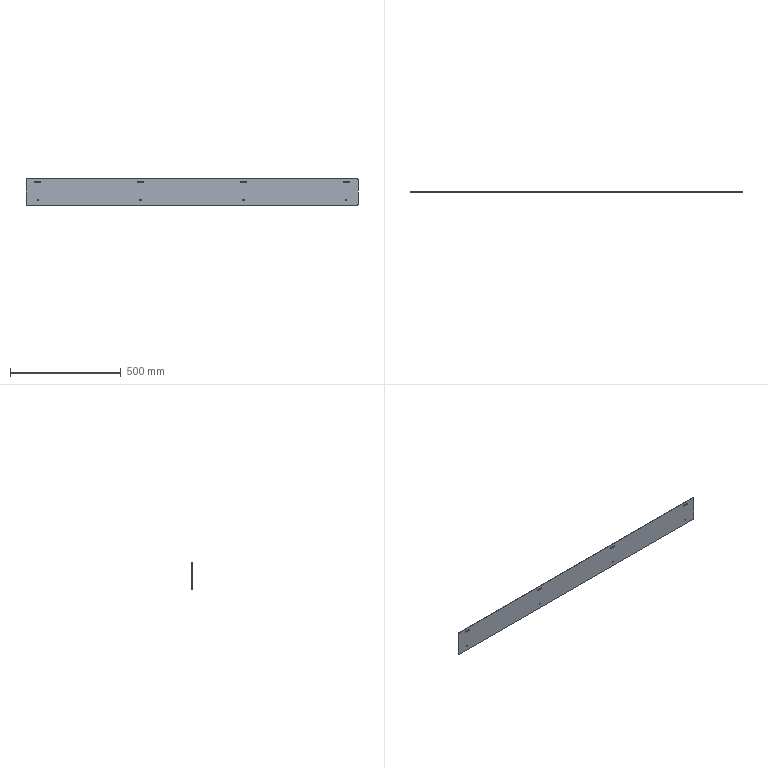Part | NX | features BREP 1 | 1 solid | 34 faces | box 1500 x 3 x 120 mm | volume 537871 mm3 | cylinder 20 | plane 14 | commonest cylinder face diameters 5.5 x8 6.004 x8 10 x4
STEP:
#1=CARTESIAN_POINT('',(-750.,0.,-55.));
#2=VERTEX_POINT('',#1);
#3=CARTESIAN_POINT('',(-750.,0.,55.));
#4=VERTEX_POINT('',#3);
#5=CARTESIAN_POINT('',(-750.,0.,-55.));
#6=DIRECTION('',(0.,0.,1.));
#7=VECTOR('',#6,1000.);
#8=LINE('',#5,#7);
#9=EDGE_CURVE('',#2,#4,#8,.T.);
#10=ORIENTED_EDGE('',*,*,#9,.T.);
#11=CARTESIAN_POINT('',(-745.,0.,60.));
#12=VERTEX_POINT('',#11);
#13=CARTESIAN_POINT('',(-745.,0.,55.));
#14=DIRECTION('',(0.,1.,0.));
#15=DIRECTION('',(-1.,0.,0.));
#16=AXIS2_PLACEMENT_3D('',#13,#14,#15);
#17=CIRCLE('',#16,5.);
#18=EDGE_CURVE('',#4,#12,#17,.T.);
#19=ORIENTED_EDGE('',*,*,#18,.T.);
#20=CARTESIAN_POINT('',(745.,0.,60.));
#21=VERTEX_POINT('',#20);
#22=CARTESIAN_POINT('',(-745.,0.,60.));
#23=DIRECTION('',(1.,0.,0.));
#24=VECTOR('',#23,1000.);
#25=LINE('',#22,#24);
#26=EDGE_CURVE('',#12,#21,#25,.T.);
#27=ORIENTED_EDGE('',*,*,#26,.T.);
#28=CARTESIAN_POINT('',(750.,0.,55.));
#29=VERTEX_POINT('',#28);
#30=CARTESIAN_POINT('',(745.,0.,55.));
#31=DIRECTION('',(0.,1.,0.));
#32=DIRECTION('',(0.,0.,1.));
#33=AXIS2_PLACEMENT_3D('',#30,#31,#32);
#34=CIRCLE('',#33,5.);
#35=EDGE_CURVE('',#21,#29,#34,.T.);
#36=ORIENTED_EDGE('',*,*,#35,.T.);
#37=CARTESIAN_POINT('',(750.,0.,-55.));
#38=VERTEX_POINT('',#37);
#39=CARTESIAN_POINT('',(750.,0.,55.));
#40=DIRECTION('',(0.,0.,-1.));
#41=VECTOR('',#40,1000.);
#42=LINE('',#39,#41);
#43=EDGE_CURVE('',#29,#38,#42,.T.);
#44=ORIENTED_EDGE('',*,*,#43,.T.);
#45=CARTESIAN_POINT('',(745.,0.,-60.));
#46=VERTEX_POINT('',#45);
#47=CARTESIAN_POINT('',(745.,0.,-55.));
#48=DIRECTION('',(0.,1.,0.));
#49=DIRECTION('',(1.,0.,0.));
#50=AXIS2_PLACEMENT_3D('',#47,#48,#49);
#51=CIRCLE('',#50,5.);
#52=EDGE_CURVE('',#38,#46,#51,.T.);
#53=ORIENTED_EDGE('',*,*,#52,.T.);
#54=CARTESIAN_POINT('',(-745.,0.,-60.));
#55=VERTEX_POINT('',#54);
#56=CARTESIAN_POINT('',(745.,0.,-60.));
#57=DIRECTION('',(-1.,0.,0.));
#58=VECTOR('',#57,1000.);
#59=LINE('',#56,#58);
#60=EDGE_CURVE('',#46,#55,#59,.T.);
#61=ORIENTED_EDGE('',*,*,#60,.T.);
#62=CARTESIAN_POINT('',(-745.,0.,-55.));
#63=DIRECTION('',(0.,1.,0.));
#64=DIRECTION('',(0.,0.,-1.));
#65=AXIS2_PLACEMENT_3D('',#62,#63,#64);
#66=CIRCLE('',#65,5.);
#67=EDGE_CURVE('',#55,#2,#66,.T.);
#68=ORIENTED_EDGE('',*,*,#67,.T.);
#69=EDGE_LOOP('',(#10,#19,#27,#36,#44,#53,#61,#68));
#70=FACE_BOUND('',#69,.T.);
#71=CARTESIAN_POINT('',(687.404,0.,48.));
#72=VERTEX_POINT('',#71);
#73=CARTESIAN_POINT('',(707.598,0.,48.));
#74=VERTEX_POINT('',#73);
#75=CARTESIAN_POINT('',(687.404,0.,48.));
#76=DIRECTION('',(1.,0.,0.));
#77=VECTOR('',#76,1000.);
#78=LINE('',#75,#77);
#79=EDGE_CURVE('',#72,#74,#78,.T.);
#80=ORIENTED_EDGE('',*,*,#79,.F.);
#81=CARTESIAN_POINT('',(687.615,0.,42.));
#82=VERTEX_POINT('',#81);
#83=CARTESIAN_POINT('',(687.5,0.,45.));
#84=DIRECTION('',(0.,-1.,0.));
#85=DIRECTION('',(-0.032,0.,0.9995));
#86=AXIS2_PLACEMENT_3D('',#83,#84,#85);
#87=CIRCLE('',#86,3.002);
#88=EDGE_CURVE('',#72,#82,#87,.T.);
#89=ORIENTED_EDGE('',*,*,#88,.T.);
#90=CARTESIAN_POINT('',(707.385,0.,42.));
#91=VERTEX_POINT('',#90);
#92=CARTESIAN_POINT('',(707.385,0.,42.));
#93=DIRECTION('',(-1.,0.,0.));
#94=VECTOR('',#93,1000.);
#95=LINE('',#92,#94);
#96=EDGE_CURVE('',#91,#82,#95,.T.);
#97=ORIENTED_EDGE('',*,*,#96,.F.);
#98=CARTESIAN_POINT('',(707.5,0.,45.));
#99=DIRECTION('',(0.,-1.,0.));
#100=DIRECTION('',(-0.03833,0.,-0.9993));
#101=AXIS2_PLACEMENT_3D('',#98,#99,#100);
#102=CIRCLE('',#101,3.002);
#103=EDGE_CURVE('',#91,#74,#102,.T.);
#104=ORIENTED_EDGE('',*,*,#103,.T.);
#105=EDGE_LOOP('',(#80,#89,#97,#104));
#106=FACE_BOUND('',#105,.T.);
#107=CARTESIAN_POINT('',(222.404,0.,48.));
#108=VERTEX_POINT('',#107);
#109=CARTESIAN_POINT('',(242.598,0.,48.));
#110=VERTEX_POINT('',#109);
#111=CARTESIAN_POINT('',(222.404,0.,48.));
#112=DIRECTION('',(1.,0.,0.));
#113=VECTOR('',#112,1000.);
#114=LINE('',#111,#113);
#115=EDGE_CURVE('',#108,#110,#114,.T.);
#116=ORIENTED_EDGE('',*,*,#115,.F.);
#117=CARTESIAN_POINT('',(222.615,0.,42.));
#118=VERTEX_POINT('',#117);
#119=CARTESIAN_POINT('',(222.5,0.,45.));
#120=DIRECTION('',(0.,-1.,0.));
#121=DIRECTION('',(-0.032,0.,0.9995));
#122=AXIS2_PLACEMENT_3D('',#119,#120,#121);
#123=CIRCLE('',#122,3.002);
#124=EDGE_CURVE('',#108,#118,#123,.T.);
#125=ORIENTED_EDGE('',*,*,#124,.T.);
#126=CARTESIAN_POINT('',(242.385,0.,42.));
#127=VERTEX_POINT('',#126);
#128=CARTESIAN_POINT('',(242.385,0.,42.));
#129=DIRECTION('',(-1.,0.,0.));
#130=VECTOR('',#129,1000.);
#131=LINE('',#128,#130);
#132=EDGE_CURVE('',#127,#118,#131,.T.);
#133=ORIENTED_EDGE('',*,*,#132,.F.);
#134=CARTESIAN_POINT('',(242.5,0.,45.));
#135=DIRECTION('',(0.,-1.,0.));
#136=DIRECTION('',(-0.03833,0.,-0.9993));
#137=AXIS2_PLACEMENT_3D('',#134,#135,#136);
#138=CIRCLE('',#137,3.002);
#139=EDGE_CURVE('',#127,#110,#138,.T.);
#140=ORIENTED_EDGE('',*,*,#139,.T.);
#141=EDGE_LOOP('',(#116,#125,#133,#140));
#142=FACE_BOUND('',#141,.T.);
#143=CARTESIAN_POINT('',(-242.596,0.,48.));
#144=VERTEX_POINT('',#143);
#145=CARTESIAN_POINT('',(-222.402,0.,48.));
#146=VERTEX_POINT('',#145);
#147=CARTESIAN_POINT('',(-242.596,0.,48.));
#148=DIRECTION('',(1.,0.,0.));
#149=VECTOR('',#148,1000.);
#150=LINE('',#147,#149);
#151=EDGE_CURVE('',#144,#146,#150,.T.);
#152=ORIENTED_EDGE('',*,*,#151,.F.);
#153=CARTESIAN_POINT('',(-242.385,0.,42.));
#154=VERTEX_POINT('',#153);
#155=CARTESIAN_POINT('',(-242.5,0.,45.));
#156=DIRECTION('',(0.,-1.,0.));
#157=DIRECTION('',(-0.032,0.,0.9995));
#158=AXIS2_PLACEMENT_3D('',#155,#156,#157);
#159=CIRCLE('',#158,3.002);
#160=EDGE_CURVE('',#144,#154,#159,.T.);
#161=ORIENTED_EDGE('',*,*,#160,.T.);
#162=CARTESIAN_POINT('',(-222.615,0.,42.));
#163=VERTEX_POINT('',#162);
#164=CARTESIAN_POINT('',(-222.615,0.,42.));
#165=DIRECTION('',(-1.,0.,0.));
#166=VECTOR('',#165,1000.);
#167=LINE('',#164,#166);
#168=EDGE_CURVE('',#163,#154,#167,.T.);
#169=ORIENTED_EDGE('',*,*,#168,.F.);
#170=CARTESIAN_POINT('',(-222.5,0.,45.));
#171=DIRECTION('',(0.,-1.,0.));
#172=DIRECTION('',(-0.03833,0.,-0.9993));
#173=AXIS2_PLACEMENT_3D('',#170,#171,#172);
#174=CIRCLE('',#173,3.002);
#175=EDGE_CURVE('',#163,#146,#174,.T.);
#176=ORIENTED_EDGE('',*,*,#175,.T.);
#177=EDGE_LOOP('',(#152,#161,#169,#176));
#178=FACE_BOUND('',#177,.T.);
#179=CARTESIAN_POINT('',(-707.596,0.,48.));
#180=VERTEX_POINT('',#179);
#181=CARTESIAN_POINT('',(-687.402,0.,48.));
#182=VERTEX_POINT('',#181);
#183=CARTESIAN_POINT('',(-707.596,0.,48.));
#184=DIRECTION('',(1.,0.,0.));
#185=VECTOR('',#184,1000.);
#186=LINE('',#183,#185);
#187=EDGE_CURVE('',#180,#182,#186,.T.);
#188=ORIENTED_EDGE('',*,*,#187,.F.);
#189=CARTESIAN_POINT('',(-707.385,0.,42.));
#190=VERTEX_POINT('',#189);
#191=CARTESIAN_POINT('',(-707.5,0.,45.));
#192=DIRECTION('',(0.,-1.,0.));
#193=DIRECTION('',(-0.032,0.,0.9995));
#194=AXIS2_PLACEMENT_3D('',#191,#192,#193);
#195=CIRCLE('',#194,3.002);
#196=EDGE_CURVE('',#180,#190,#195,.T.);
#197=ORIENTED_EDGE('',*,*,#196,.T.);
#198=CARTESIAN_POINT('',(-687.615,0.,42.));
#199=VERTEX_POINT('',#198);
#200=CARTESIAN_POINT('',(-687.615,0.,42.));
#201=DIRECTION('',(-1.,0.,0.));
#202=VECTOR('',#201,1000.);
#203=LINE('',#200,#202);
#204=EDGE_CURVE('',#199,#190,#203,.T.);
#205=ORIENTED_EDGE('',*,*,#204,.F.);
#206=CARTESIAN_POINT('',(-687.5,0.,45.));
#207=DIRECTION('',(0.,-1.,0.));
#208=DIRECTION('',(-0.03833,0.,-0.9993));
#209=AXIS2_PLACEMENT_3D('',#206,#207,#208);
#210=CIRCLE('',#209,3.002);
#211=EDGE_CURVE('',#199,#182,#210,.T.);
#212=ORIENTED_EDGE('',*,*,#211,.T.);
#213=EDGE_LOOP('',(#188,#197,#205,#212));
#214=FACE_BOUND('',#213,.T.);
#215=CARTESIAN_POINT('',(700.25,0.,-36.));
#216=VERTEX_POINT('',#215);
#217=CARTESIAN_POINT('',(694.75,0.,-36.));
#218=VERTEX_POINT('',#217);
#219=CARTESIAN_POINT('',(697.5,0.,-36.));
#220=DIRECTION('',(0.,-1.,0.));
#221=DIRECTION('',(1.,0.,0.));
#222=AXIS2_PLACEMENT_3D('',#219,#220,#221);
#223=CIRCLE('',#222,2.75);
#224=EDGE_CURVE('',#216,#218,#223,.T.);
#225=ORIENTED_EDGE('',*,*,#224,.T.);
#226=CARTESIAN_POINT('',(697.5,0.,-36.));
#227=DIRECTION('',(0.,-1.,0.));
#228=DIRECTION('',(-1.,0.,0.));
#229=AXIS2_PLACEMENT_3D('',#226,#227,#228);
#230=CIRCLE('',#229,2.75);
#231=EDGE_CURVE('',#218,#216,#230,.T.);
#232=ORIENTED_EDGE('',*,*,#231,.T.);
#233=EDGE_LOOP('',(#225,#232));
#234=FACE_BOUND('',#233,.T.);
#235=CARTESIAN_POINT('',(235.25,0.,-36.));
#236=VERTEX_POINT('',#235);
#237=CARTESIAN_POINT('',(229.75,0.,-36.));
#238=VERTEX_POINT('',#237);
#239=CARTESIAN_POINT('',(232.5,0.,-36.));
#240=DIRECTION('',(0.,-1.,0.));
#241=DIRECTION('',(1.,0.,0.));
#242=AXIS2_PLACEMENT_3D('',#239,#240,#241);
#243=CIRCLE('',#242,2.75);
#244=EDGE_CURVE('',#236,#238,#243,.T.);
#245=ORIENTED_EDGE('',*,*,#244,.T.);
#246=CARTESIAN_POINT('',(232.5,0.,-36.));
#247=DIRECTION('',(0.,-1.,0.));
#248=DIRECTION('',(-1.,0.,0.));
#249=AXIS2_PLACEMENT_3D('',#246,#247,#248);
#250=CIRCLE('',#249,2.75);
#251=EDGE_CURVE('',#238,#236,#250,.T.);
#252=ORIENTED_EDGE('',*,*,#251,.T.);
#253=EDGE_LOOP('',(#245,#252));
#254=FACE_BOUND('',#253,.T.);
#255=CARTESIAN_POINT('',(-229.75,0.,-36.));
#256=VERTEX_POINT('',#255);
#257=CARTESIAN_POINT('',(-235.25,0.,-36.));
#258=VERTEX_POINT('',#257);
#259=CARTESIAN_POINT('',(-232.5,0.,-36.));
#260=DIRECTION('',(0.,-1.,0.));
#261=DIRECTION('',(1.,0.,0.));
#262=AXIS2_PLACEMENT_3D('',#259,#260,#261);
#263=CIRCLE('',#262,2.75);
#264=EDGE_CURVE('',#256,#258,#263,.T.);
#265=ORIENTED_EDGE('',*,*,#264,.T.);
#266=CARTESIAN_POINT('',(-232.5,0.,-36.));
#267=DIRECTION('',(0.,-1.,0.));
#268=DIRECTION('',(-1.,0.,0.));
#269=AXIS2_PLACEMENT_3D('',#266,#267,#268);
#270=CIRCLE('',#269,2.75);
#271=EDGE_CURVE('',#258,#256,#270,.T.);
#272=ORIENTED_EDGE('',*,*,#271,.T.);
#273=EDGE_LOOP('',(#265,#272));
#274=FACE_BOUND('',#273,.T.);
#275=CARTESIAN_POINT('',(-694.75,0.,-36.));
#276=VERTEX_POINT('',#275);
#277=CARTESIAN_POINT('',(-700.25,0.,-36.));
#278=VERTEX_POINT('',#277);
#279=CARTESIAN_POINT('',(-697.5,0.,-36.));
#280=DIRECTION('',(0.,-1.,0.));
#281=DIRECTION('',(1.,0.,0.));
#282=AXIS2_PLACEMENT_3D('',#279,#280,#281);
#283=CIRCLE('',#282,2.75);
#284=EDGE_CURVE('',#276,#278,#283,.T.);
#285=ORIENTED_EDGE('',*,*,#284,.T.);
#286=CARTESIAN_POINT('',(-697.5,0.,-36.));
#287=DIRECTION('',(0.,-1.,0.));
#288=DIRECTION('',(-1.,0.,0.));
#289=AXIS2_PLACEMENT_3D('',#286,#287,#288);
#290=CIRCLE('',#289,2.75);
#291=EDGE_CURVE('',#278,#276,#290,.T.);
#292=ORIENTED_EDGE('',*,*,#291,.T.);
#293=EDGE_LOOP('',(#285,#292));
#294=FACE_BOUND('',#293,.T.);
#295=CARTESIAN_POINT('',(0.,0.,0.));
#296=DIRECTION('',(0.,1.,0.));
#297=DIRECTION('',(1.,0.,0.));
#298=AXIS2_PLACEMENT_3D('',#295,#296,#297);
#299=PLANE('',#298);
#300=ADVANCED_FACE('',(#70,#106,#142,#178,#214,#234,#254,#274,#294),#299,.T.);
#301=CARTESIAN_POINT('',(-745.,-3.,-60.));
#302=VERTEX_POINT('',#301);
#303=CARTESIAN_POINT('',(-745.,-3.,-60.));
#304=DIRECTION('',(0.,1.,0.));
#305=VECTOR('',#304,1000.);
#306=LINE('',#303,#305);
#307=EDGE_CURVE('',#302,#55,#306,.T.);
#308=ORIENTED_EDGE('',*,*,#307,.F.);
#309=CARTESIAN_POINT('',(-750.,-3.,-55.));
#310=VERTEX_POINT('',#309);
#311=CARTESIAN_POINT('',(-745.,-3.,-55.));
#312=DIRECTION('',(0.,-1.,0.));
#313=DIRECTION('',(-1.,0.,0.));
#314=AXIS2_PLACEMENT_3D('',#311,#312,#313);
#315=CIRCLE('',#314,5.);
#316=EDGE_CURVE('',#310,#302,#315,.T.);
#317=ORIENTED_EDGE('',*,*,#316,.F.);
#318=CARTESIAN_POINT('',(-750.,-3.,-55.));
#319=DIRECTION('',(0.,1.,0.));
#320=VECTOR('',#319,1000.);
#321=LINE('',#318,#320);
#322=EDGE_CURVE('',#310,#2,#321,.T.);
#323=ORIENTED_EDGE('',*,*,#322,.T.);
#324=ORIENTED_EDGE('',*,*,#67,.F.);
#325=EDGE_LOOP('',(#308,#317,#323,#324));
#326=FACE_BOUND('',#325,.T.);
#327=CARTESIAN_POINT('',(-745.,-9.316,-55.));
#328=DIRECTION('',(0.,1.,0.));
#329=DIRECTION('',(0.,0.,-1.));
#330=AXIS2_PLACEMENT_3D('',#327,#328,#329);
#331=CYLINDRICAL_SURFACE('',#330,5.);
#332=ADVANCED_FACE('',(#326),#331,.T.);
#333=CARTESIAN_POINT('',(-750.,-3.,55.));
#334=VERTEX_POINT('',#333);
#335=CARTESIAN_POINT('',(-750.,-3.,-55.));
#336=DIRECTION('',(0.,0.,1.));
#337=VECTOR('',#336,1000.);
#338=LINE('',#335,#337);
#339=EDGE_CURVE('',#310,#334,#338,.T.);
#340=ORIENTED_EDGE('',*,*,#339,.T.);
#341=CARTESIAN_POINT('',(-750.,-3.,55.));
#342=DIRECTION('',(0.,1.,0.));
#343=VECTOR('',#342,1000.);
#344=LINE('',#341,#343);
#345=EDGE_CURVE('',#334,#4,#344,.T.);
#346=ORIENTED_EDGE('',*,*,#345,.T.);
#347=ORIENTED_EDGE('',*,*,#9,.F.);
#348=ORIENTED_EDGE('',*,*,#322,.F.);
#349=EDGE_LOOP('',(#340,#346,#347,#348));
#350=FACE_BOUND('',#349,.T.);
#351=CARTESIAN_POINT('',(-750.,-1.5,0.));
#352=DIRECTION('',(-1.,0.,0.));
#353=DIRECTION('',(0.,0.,1.));
#354=AXIS2_PLACEMENT_3D('',#351,#352,#353);
#355=PLANE('',#354);
#356=ADVANCED_FACE('',(#350),#355,.T.);
#357=ORIENTED_EDGE('',*,*,#345,.F.);
#358=CARTESIAN_POINT('',(-745.,-3.,60.));
#359=VERTEX_POINT('',#358);
#360=CARTESIAN_POINT('',(-745.,-3.,55.));
#361=DIRECTION('',(0.,-1.,0.));
#362=DIRECTION('',(0.,0.,1.));
#363=AXIS2_PLACEMENT_3D('',#360,#361,#362);
#364=CIRCLE('',#363,5.);
#365=EDGE_CURVE('',#359,#334,#364,.T.);
#366=ORIENTED_EDGE('',*,*,#365,.F.);
#367=CARTESIAN_POINT('',(-745.,-3.,60.));
#368=DIRECTION('',(0.,1.,0.));
#369=VECTOR('',#368,1000.);
#370=LINE('',#367,#369);
#371=EDGE_CURVE('',#359,#12,#370,.T.);
#372=ORIENTED_EDGE('',*,*,#371,.T.);
#373=ORIENTED_EDGE('',*,*,#18,.F.);
#374=EDGE_LOOP('',(#357,#366,#372,#373));
#375=FACE_BOUND('',#374,.T.);
#376=CARTESIAN_POINT('',(-745.,-9.316,55.));
#377=DIRECTION('',(0.,1.,0.));
#378=DIRECTION('',(-1.,0.,0.));
#379=AXIS2_PLACEMENT_3D('',#376,#377,#378);
#380=CYLINDRICAL_SURFACE('',#379,5.);
#381=ADVANCED_FACE('',(#375),#380,.T.);
#382=CARTESIAN_POINT('',(745.,-3.,60.));
#383=VERTEX_POINT('',#382);
#384=CARTESIAN_POINT('',(-745.,-3.,60.));
#385=DIRECTION('',(1.,0.,0.));
#386=VECTOR('',#385,1000.);
#387=LINE('',#384,#386);
#388=EDGE_CURVE('',#359,#383,#387,.T.);
#389=ORIENTED_EDGE('',*,*,#388,.T.);
#390=CARTESIAN_POINT('',(745.,-3.,60.));
#391=DIRECTION('',(0.,1.,0.));
#392=VECTOR('',#391,1000.);
#393=LINE('',#390,#392);
#394=EDGE_CURVE('',#383,#21,#393,.T.);
#395=ORIENTED_EDGE('',*,*,#394,.T.);
#396=ORIENTED_EDGE('',*,*,#26,.F.);
#397=ORIENTED_EDGE('',*,*,#371,.F.);
#398=EDGE_LOOP('',(#389,#395,#396,#397));
#399=FACE_BOUND('',#398,.T.);
#400=CARTESIAN_POINT('',(0.,-1.5,60.));
#401=DIRECTION('',(0.,0.,1.));
#402=DIRECTION('',(1.,0.,0.));
#403=AXIS2_PLACEMENT_3D('',#400,#401,#402);
#404=PLANE('',#403);
#405=ADVANCED_FACE('',(#399),#404,.T.);
#406=ORIENTED_EDGE('',*,*,#394,.F.);
#407=CARTESIAN_POINT('',(750.,-3.,55.));
#408=VERTEX_POINT('',#407);
#409=CARTESIAN_POINT('',(745.,-3.,55.));
#410=DIRECTION('',(0.,-1.,0.));
#411=DIRECTION('',(1.,0.,0.));
#412=AXIS2_PLACEMENT_3D('',#409,#410,#411);
#413=CIRCLE('',#412,5.);
#414=EDGE_CURVE('',#408,#383,#413,.T.);
#415=ORIENTED_EDGE('',*,*,#414,.F.);
#416=CARTESIAN_POINT('',(750.,-3.,55.));
#417=DIRECTION('',(0.,1.,0.));
#418=VECTOR('',#417,1000.);
#419=LINE('',#416,#418);
#420=EDGE_CURVE('',#408,#29,#419,.T.);
#421=ORIENTED_EDGE('',*,*,#420,.T.);
#422=ORIENTED_EDGE('',*,*,#35,.F.);
#423=EDGE_LOOP('',(#406,#415,#421,#422));
#424=FACE_BOUND('',#423,.T.);
#425=CARTESIAN_POINT('',(745.,-9.316,55.));
#426=DIRECTION('',(0.,1.,0.));
#427=DIRECTION('',(0.,0.,1.));
#428=AXIS2_PLACEMENT_3D('',#425,#426,#427);
#429=CYLINDRICAL_SURFACE('',#428,5.);
#430=ADVANCED_FACE('',(#424),#429,.T.);
#431=ORIENTED_EDGE('',*,*,#43,.F.);
#432=ORIENTED_EDGE('',*,*,#420,.F.);
#433=CARTESIAN_POINT('',(750.,-3.,-55.));
#434=VERTEX_POINT('',#433);
#435=CARTESIAN_POINT('',(750.,-3.,55.));
#436=DIRECTION('',(0.,0.,-1.));
#437=VECTOR('',#436,1000.);
#438=LINE('',#435,#437);
#439=EDGE_CURVE('',#408,#434,#438,.T.);
#440=ORIENTED_EDGE('',*,*,#439,.T.);
#441=CARTESIAN_POINT('',(750.,-3.,-55.));
#442=DIRECTION('',(0.,1.,0.));
#443=VECTOR('',#442,1000.);
#444=LINE('',#441,#443);
#445=EDGE_CURVE('',#434,#38,#444,.T.);
#446=ORIENTED_EDGE('',*,*,#445,.T.);
#447=EDGE_LOOP('',(#431,#432,#440,#446));
#448=FACE_BOUND('',#447,.T.);
#449=CARTESIAN_POINT('',(750.,-1.5,0.));
#450=DIRECTION('',(1.,0.,0.));
#451=DIRECTION('',(0.,1.,0.));
#452=AXIS2_PLACEMENT_3D('',#449,#450,#451);
#453=PLANE('',#452);
#454=ADVANCED_FACE('',(#448),#453,.T.);
#455=ORIENTED_EDGE('',*,*,#445,.F.);
#456=CARTESIAN_POINT('',(745.,-3.,-60.));
#457=VERTEX_POINT('',#456);
#458=CARTESIAN_POINT('',(745.,-3.,-55.));
#459=DIRECTION('',(0.,-1.,0.));
#460=DIRECTION('',(0.,0.,-1.));
#461=AXIS2_PLACEMENT_3D('',#458,#459,#460);
#462=CIRCLE('',#461,5.);
#463=EDGE_CURVE('',#457,#434,#462,.T.);
#464=ORIENTED_EDGE('',*,*,#463,.F.);
#465=CARTESIAN_POINT('',(745.,-3.,-60.));
#466=DIRECTION('',(0.,1.,0.));
#467=VECTOR('',#466,1000.);
#468=LINE('',#465,#467);
#469=EDGE_CURVE('',#457,#46,#468,.T.);
#470=ORIENTED_EDGE('',*,*,#469,.T.);
#471=ORIENTED_EDGE('',*,*,#52,.F.);
#472=EDGE_LOOP('',(#455,#464,#470,#471));
#473=FACE_BOUND('',#472,.T.);
#474=CARTESIAN_POINT('',(745.,-9.316,-55.));
#475=DIRECTION('',(0.,1.,0.));
#476=DIRECTION('',(1.,0.,0.));
#477=AXIS2_PLACEMENT_3D('',#474,#475,#476);
#478=CYLINDRICAL_SURFACE('',#477,5.);
#479=ADVANCED_FACE('',(#473),#478,.T.);
#480=ORIENTED_EDGE('',*,*,#60,.F.);
#481=ORIENTED_EDGE('',*,*,#469,.F.);
#482=CARTESIAN_POINT('',(745.,-3.,-60.));
#483=DIRECTION('',(-1.,0.,0.));
#484=VECTOR('',#483,1000.);
#485=LINE('',#482,#484);
#486=EDGE_CURVE('',#457,#302,#485,.T.);
#487=ORIENTED_EDGE('',*,*,#486,.T.);
#488=ORIENTED_EDGE('',*,*,#307,.T.);
#489=EDGE_LOOP('',(#480,#481,#487,#488));
#490=FACE_BOUND('',#489,.T.);
#491=CARTESIAN_POINT('',(0.,-1.5,-60.));
#492=DIRECTION('',(0.,0.,-1.));
#493=DIRECTION('',(0.,-1.,0.));
#494=AXIS2_PLACEMENT_3D('',#491,#492,#493);
#495=PLANE('',#494);
#496=ADVANCED_FACE('',(#490),#495,.T.);
#497=ORIENTED_EDGE('',*,*,#486,.F.);
#498=ORIENTED_EDGE('',*,*,#463,.T.);
#499=ORIENTED_EDGE('',*,*,#439,.F.);
#500=ORIENTED_EDGE('',*,*,#414,.T.);
#501=ORIENTED_EDGE('',*,*,#388,.F.);
#502=ORIENTED_EDGE('',*,*,#365,.T.);
#503=ORIENTED_EDGE('',*,*,#339,.F.);
#504=ORIENTED_EDGE('',*,*,#316,.T.);
#505=EDGE_LOOP('',(#497,#498,#499,#500,#501,#502,#503,#504));
#506=FACE_BOUND('',#505,.T.);
#507=CARTESIAN_POINT('',(707.385,-3.,42.));
#508=VERTEX_POINT('',#507);
#509=CARTESIAN_POINT('',(687.615,-3.,42.));
#510=VERTEX_POINT('',#509);
#511=CARTESIAN_POINT('',(707.385,-3.,42.));
#512=DIRECTION('',(-1.,0.,0.));
#513=VECTOR('',#512,1000.);
#514=LINE('',#511,#513);
#515=EDGE_CURVE('',#508,#510,#514,.T.);
#516=ORIENTED_EDGE('',*,*,#515,.T.);
#517=CARTESIAN_POINT('',(687.404,-3.,48.));
#518=VERTEX_POINT('',#517);
#519=CARTESIAN_POINT('',(687.5,-3.,45.));
#520=DIRECTION('',(0.,-1.,0.));
#521=DIRECTION('',(-0.032,0.,0.9995));
#522=AXIS2_PLACEMENT_3D('',#519,#520,#521);
#523=CIRCLE('',#522,3.002);
#524=EDGE_CURVE('',#518,#510,#523,.T.);
#525=ORIENTED_EDGE('',*,*,#524,.F.);
#526=CARTESIAN_POINT('',(707.598,-3.,48.));
#527=VERTEX_POINT('',#526);
#528=CARTESIAN_POINT('',(687.404,-3.,48.));
#529=DIRECTION('',(1.,0.,0.));
#530=VECTOR('',#529,1000.);
#531=LINE('',#528,#530);
#532=EDGE_CURVE('',#518,#527,#531,.T.);
#533=ORIENTED_EDGE('',*,*,#532,.T.);
#534=CARTESIAN_POINT('',(707.5,-3.,45.));
#535=DIRECTION('',(0.,-1.,0.));
#536=DIRECTION('',(-0.03833,0.,-0.9993));
#537=AXIS2_PLACEMENT_3D('',#534,#535,#536);
#538=CIRCLE('',#537,3.002);
#539=EDGE_CURVE('',#508,#527,#538,.T.);
#540=ORIENTED_EDGE('',*,*,#539,.F.);
#541=EDGE_LOOP('',(#516,#525,#533,#540));
#542=FACE_BOUND('',#541,.T.);
#543=CARTESIAN_POINT('',(242.385,-3.,42.));
#544=VERTEX_POINT('',#543);
#545=CARTESIAN_POINT('',(222.615,-3.,42.));
#546=VERTEX_POINT('',#545);
#547=CARTESIAN_POINT('',(242.385,-3.,42.));
#548=DIRECTION('',(-1.,0.,0.));
#549=VECTOR('',#548,1000.);
#550=LINE('',#547,#549);
#551=EDGE_CURVE('',#544,#546,#550,.T.);
#552=ORIENTED_EDGE('',*,*,#551,.T.);
#553=CARTESIAN_POINT('',(222.404,-3.,48.));
#554=VERTEX_POINT('',#553);
#555=CARTESIAN_POINT('',(222.5,-3.,45.));
#556=DIRECTION('',(0.,-1.,0.));
#557=DIRECTION('',(-0.032,0.,0.9995));
#558=AXIS2_PLACEMENT_3D('',#555,#556,#557);
#559=CIRCLE('',#558,3.002);
#560=EDGE_CURVE('',#554,#546,#559,.T.);
#561=ORIENTED_EDGE('',*,*,#560,.F.);
#562=CARTESIAN_POINT('',(242.598,-3.,48.));
#563=VERTEX_POINT('',#562);
#564=CARTESIAN_POINT('',(222.404,-3.,48.));
#565=DIRECTION('',(1.,0.,0.));
#566=VECTOR('',#565,1000.);
#567=LINE('',#564,#566);
#568=EDGE_CURVE('',#554,#563,#567,.T.);
#569=ORIENTED_EDGE('',*,*,#568,.T.);
#570=CARTESIAN_POINT('',(242.5,-3.,45.));
#571=DIRECTION('',(0.,-1.,0.));
#572=DIRECTION('',(-0.03833,0.,-0.9993));
#573=AXIS2_PLACEMENT_3D('',#570,#571,#572);
#574=CIRCLE('',#573,3.002);
#575=EDGE_CURVE('',#544,#563,#574,.T.);
#576=ORIENTED_EDGE('',*,*,#575,.F.);
#577=EDGE_LOOP('',(#552,#561,#569,#576));
#578=FACE_BOUND('',#577,.T.);
#579=CARTESIAN_POINT('',(-222.615,-3.,42.));
#580=VERTEX_POINT('',#579);
#581=CARTESIAN_POINT('',(-242.385,-3.,42.));
#582=VERTEX_POINT('',#581);
#583=CARTESIAN_POINT('',(-222.615,-3.,42.));
#584=DIRECTION('',(-1.,0.,0.));
#585=VECTOR('',#584,1000.);
#586=LINE('',#583,#585);
#587=EDGE_CURVE('',#580,#582,#586,.T.);
#588=ORIENTED_EDGE('',*,*,#587,.T.);
#589=CARTESIAN_POINT('',(-242.596,-3.,48.));
#590=VERTEX_POINT('',#589);
#591=CARTESIAN_POINT('',(-242.5,-3.,45.));
#592=DIRECTION('',(0.,-1.,0.));
#593=DIRECTION('',(-0.032,0.,0.9995));
#594=AXIS2_PLACEMENT_3D('',#591,#592,#593);
#595=CIRCLE('',#594,3.002);
#596=EDGE_CURVE('',#590,#582,#595,.T.);
#597=ORIENTED_EDGE('',*,*,#596,.F.);
#598=CARTESIAN_POINT('',(-222.402,-3.,48.));
#599=VERTEX_POINT('',#598);
#600=CARTESIAN_POINT('',(-242.596,-3.,48.));
#601=DIRECTION('',(1.,0.,0.));
#602=VECTOR('',#601,1000.);
#603=LINE('',#600,#602);
#604=EDGE_CURVE('',#590,#599,#603,.T.);
#605=ORIENTED_EDGE('',*,*,#604,.T.);
#606=CARTESIAN_POINT('',(-222.5,-3.,45.));
#607=DIRECTION('',(0.,-1.,0.));
#608=DIRECTION('',(-0.03833,0.,-0.9993));
#609=AXIS2_PLACEMENT_3D('',#606,#607,#608);
#610=CIRCLE('',#609,3.002);
#611=EDGE_CURVE('',#580,#599,#610,.T.);
#612=ORIENTED_EDGE('',*,*,#611,.F.);
#613=EDGE_LOOP('',(#588,#597,#605,#612));
#614=FACE_BOUND('',#613,.T.);
#615=CARTESIAN_POINT('',(-687.615,-3.,42.));
#616=VERTEX_POINT('',#615);
#617=CARTESIAN_POINT('',(-707.385,-3.,42.));
#618=VERTEX_POINT('',#617);
#619=CARTESIAN_POINT('',(-687.615,-3.,42.));
#620=DIRECTION('',(-1.,0.,0.));
#621=VECTOR('',#620,1000.);
#622=LINE('',#619,#621);
#623=EDGE_CURVE('',#616,#618,#622,.T.);
#624=ORIENTED_EDGE('',*,*,#623,.T.);
#625=CARTESIAN_POINT('',(-707.596,-3.,48.));
#626=VERTEX_POINT('',#625);
#627=CARTESIAN_POINT('',(-707.5,-3.,45.));
#628=DIRECTION('',(0.,-1.,0.));
#629=DIRECTION('',(-0.032,0.,0.9995));
#630=AXIS2_PLACEMENT_3D('',#627,#628,#629);
#631=CIRCLE('',#630,3.002);
#632=EDGE_CURVE('',#626,#618,#631,.T.);
#633=ORIENTED_EDGE('',*,*,#632,.F.);
#634=CARTESIAN_POINT('',(-687.402,-3.,48.));
#635=VERTEX_POINT('',#634);
#636=CARTESIAN_POINT('',(-707.596,-3.,48.));
#637=DIRECTION('',(1.,0.,0.));
#638=VECTOR('',#637,1000.);
#639=LINE('',#636,#638);
#640=EDGE_CURVE('',#626,#635,#639,.T.);
#641=ORIENTED_EDGE('',*,*,#640,.T.);
#642=CARTESIAN_POINT('',(-687.5,-3.,45.));
#643=DIRECTION('',(0.,-1.,0.));
#644=DIRECTION('',(-0.03833,0.,-0.9993));
#645=AXIS2_PLACEMENT_3D('',#642,#643,#644);
#646=CIRCLE('',#645,3.002);
#647=EDGE_CURVE('',#616,#635,#646,.T.);
#648=ORIENTED_EDGE('',*,*,#647,.F.);
#649=EDGE_LOOP('',(#624,#633,#641,#648));
#650=FACE_BOUND('',#649,.T.);
#651=CARTESIAN_POINT('',(700.25,-3.,-36.));
#652=VERTEX_POINT('',#651);
#653=CARTESIAN_POINT('',(694.75,-3.,-36.));
#654=VERTEX_POINT('',#653);
#655=CARTESIAN_POINT('',(697.5,-3.,-36.));
#656=DIRECTION('',(0.,-1.,0.));
#657=DIRECTION('',(1.,0.,0.));
#658=AXIS2_PLACEMENT_3D('',#655,#656,#657);
#659=CIRCLE('',#658,2.75);
#660=EDGE_CURVE('',#652,#654,#659,.T.);
#661=ORIENTED_EDGE('',*,*,#660,.F.);
#662=CARTESIAN_POINT('',(697.5,-3.,-36.));
#663=DIRECTION('',(0.,-1.,0.));
#664=DIRECTION('',(-1.,0.,0.));
#665=AXIS2_PLACEMENT_3D('',#662,#663,#664);
#666=CIRCLE('',#665,2.75);
#667=EDGE_CURVE('',#654,#652,#666,.T.);
#668=ORIENTED_EDGE('',*,*,#667,.F.);
#669=EDGE_LOOP('',(#661,#668));
#670=FACE_BOUND('',#669,.T.);
#671=CARTESIAN_POINT('',(235.25,-3.,-36.));
#672=VERTEX_POINT('',#671);
#673=CARTESIAN_POINT('',(229.75,-3.,-36.));
#674=VERTEX_POINT('',#673);
#675=CARTESIAN_POINT('',(232.5,-3.,-36.));
#676=DIRECTION('',(0.,-1.,0.));
#677=DIRECTION('',(1.,0.,0.));
#678=AXIS2_PLACEMENT_3D('',#675,#676,#677);
#679=CIRCLE('',#678,2.75);
#680=EDGE_CURVE('',#672,#674,#679,.T.);
#681=ORIENTED_EDGE('',*,*,#680,.F.);
#682=CARTESIAN_POINT('',(232.5,-3.,-36.));
#683=DIRECTION('',(0.,-1.,0.));
#684=DIRECTION('',(-1.,0.,0.));
#685=AXIS2_PLACEMENT_3D('',#682,#683,#684);
#686=CIRCLE('',#685,2.75);
#687=EDGE_CURVE('',#674,#672,#686,.T.);
#688=ORIENTED_EDGE('',*,*,#687,.F.);
#689=EDGE_LOOP('',(#681,#688));
#690=FACE_BOUND('',#689,.T.);
#691=CARTESIAN_POINT('',(-229.75,-3.,-36.));
#692=VERTEX_POINT('',#691);
#693=CARTESIAN_POINT('',(-235.25,-3.,-36.));
#694=VERTEX_POINT('',#693);
#695=CARTESIAN_POINT('',(-232.5,-3.,-36.));
#696=DIRECTION('',(0.,-1.,0.));
#697=DIRECTION('',(1.,0.,0.));
#698=AXIS2_PLACEMENT_3D('',#695,#696,#697);
#699=CIRCLE('',#698,2.75);
#700=EDGE_CURVE('',#692,#694,#699,.T.);
#701=ORIENTED_EDGE('',*,*,#700,.F.);
#702=CARTESIAN_POINT('',(-232.5,-3.,-36.));
#703=DIRECTION('',(0.,-1.,0.));
#704=DIRECTION('',(-1.,0.,0.));
#705=AXIS2_PLACEMENT_3D('',#702,#703,#704);
#706=CIRCLE('',#705,2.75);
#707=EDGE_CURVE('',#694,#692,#706,.T.);
#708=ORIENTED_EDGE('',*,*,#707,.F.);
#709=EDGE_LOOP('',(#701,#708));
#710=FACE_BOUND('',#709,.T.);
#711=CARTESIAN_POINT('',(-694.75,-3.,-36.));
#712=VERTEX_POINT('',#711);
#713=CARTESIAN_POINT('',(-700.25,-3.,-36.));
#714=VERTEX_POINT('',#713);
#715=CARTESIAN_POINT('',(-697.5,-3.,-36.));
#716=DIRECTION('',(0.,-1.,0.));
#717=DIRECTION('',(1.,0.,0.));
#718=AXIS2_PLACEMENT_3D('',#715,#716,#717);
#719=CIRCLE('',#718,2.75);
#720=EDGE_CURVE('',#712,#714,#719,.T.);
#721=ORIENTED_EDGE('',*,*,#720,.F.);
#722=CARTESIAN_POINT('',(-697.5,-3.,-36.));
#723=DIRECTION('',(0.,-1.,0.));
#724=DIRECTION('',(-1.,0.,0.));
#725=AXIS2_PLACEMENT_3D('',#722,#723,#724);
#726=CIRCLE('',#725,2.75);
#727=EDGE_CURVE('',#714,#712,#726,.T.);
#728=ORIENTED_EDGE('',*,*,#727,.F.);
#729=EDGE_LOOP('',(#721,#728));
#730=FACE_BOUND('',#729,.T.);
#731=CARTESIAN_POINT('',(0.,-3.,0.));
#732=DIRECTION('',(0.,1.,0.));
#733=DIRECTION('',(1.,0.,0.));
#734=AXIS2_PLACEMENT_3D('',#731,#732,#733);
#735=PLANE('',#734);
#736=ADVANCED_FACE('',(#506,#542,#578,#614,#650,#670,#690,#710,#730),#735,.F.);
#737=CARTESIAN_POINT('',(707.385,0.,42.));
#738=DIRECTION('',(0.,-1.,0.));
#739=VECTOR('',#738,1000.);
#740=LINE('',#737,#739);
#741=EDGE_CURVE('',#91,#508,#740,.T.);
#742=ORIENTED_EDGE('',*,*,#741,.T.);
#743=ORIENTED_EDGE('',*,*,#539,.T.);
#744=CARTESIAN_POINT('',(707.598,0.,48.));
#745=DIRECTION('',(0.,-1.,0.));
#746=VECTOR('',#745,1000.);
#747=LINE('',#744,#746);
#748=EDGE_CURVE('',#74,#527,#747,.T.);
#749=ORIENTED_EDGE('',*,*,#748,.F.);
#750=ORIENTED_EDGE('',*,*,#103,.F.);
#751=EDGE_LOOP('',(#742,#743,#749,#750));
#752=FACE_BOUND('',#751,.T.);
#753=CARTESIAN_POINT('',(707.5,-1.5,45.));
#754=DIRECTION('',(0.,-1.,0.));
#755=DIRECTION('',(-0.03833,0.,-0.9993));
#756=AXIS2_PLACEMENT_3D('',#753,#754,#755);
#757=CYLINDRICAL_SURFACE('',#756,3.002);
#758=ADVANCED_FACE('',(#752),#757,.F.);
#759=ORIENTED_EDGE('',*,*,#748,.T.);
#760=ORIENTED_EDGE('',*,*,#532,.F.);
#761=CARTESIAN_POINT('',(687.404,0.,48.));
#762=DIRECTION('',(0.,-1.,0.));
#763=VECTOR('',#762,1000.);
#764=LINE('',#761,#763);
#765=EDGE_CURVE('',#72,#518,#764,.T.);
#766=ORIENTED_EDGE('',*,*,#765,.F.);
#767=ORIENTED_EDGE('',*,*,#79,.T.);
#768=EDGE_LOOP('',(#759,#760,#766,#767));
#769=FACE_BOUND('',#768,.T.);
#770=CARTESIAN_POINT('',(697.501,-1.5,48.));
#771=DIRECTION('',(0.,0.,1.));
#772=DIRECTION('',(1.,0.,0.));
#773=AXIS2_PLACEMENT_3D('',#770,#771,#772);
#774=PLANE('',#773);
#775=ADVANCED_FACE('',(#769),#774,.F.);
#776=ORIENTED_EDGE('',*,*,#765,.T.);
#777=ORIENTED_EDGE('',*,*,#524,.T.);
#778=CARTESIAN_POINT('',(687.615,0.,42.));
#779=DIRECTION('',(0.,-1.,0.));
#780=VECTOR('',#779,1000.);
#781=LINE('',#778,#780);
#782=EDGE_CURVE('',#82,#510,#781,.T.);
#783=ORIENTED_EDGE('',*,*,#782,.F.);
#784=ORIENTED_EDGE('',*,*,#88,.F.);
#785=EDGE_LOOP('',(#776,#777,#783,#784));
#786=FACE_BOUND('',#785,.T.);
#787=CARTESIAN_POINT('',(687.5,-1.5,45.));
#788=DIRECTION('',(0.,-1.,0.));
#789=DIRECTION('',(-0.032,0.,0.9995));
#790=AXIS2_PLACEMENT_3D('',#787,#788,#789);
#791=CYLINDRICAL_SURFACE('',#790,3.002);
#792=ADVANCED_FACE('',(#786),#791,.F.);
#793=ORIENTED_EDGE('',*,*,#782,.T.);
#794=ORIENTED_EDGE('',*,*,#515,.F.);
#795=ORIENTED_EDGE('',*,*,#741,.F.);
#796=ORIENTED_EDGE('',*,*,#96,.T.);
#797=EDGE_LOOP('',(#793,#794,#795,#796));
#798=FACE_BOUND('',#797,.T.);
#799=CARTESIAN_POINT('',(697.5,-1.5,42.));
#800=DIRECTION('',(0.,0.,-1.));
#801=DIRECTION('',(0.,-1.,0.));
#802=AXIS2_PLACEMENT_3D('',#799,#800,#801);
#803=PLANE('',#802);
#804=ADVANCED_FACE('',(#798),#803,.F.);
#805=CARTESIAN_POINT('',(242.385,0.,42.));
#806=DIRECTION('',(0.,-1.,0.));
#807=VECTOR('',#806,1000.);
#808=LINE('',#805,#807);
#809=EDGE_CURVE('',#127,#544,#808,.T.);
#810=ORIENTED_EDGE('',*,*,#809,.T.);
#811=ORIENTED_EDGE('',*,*,#575,.T.);
#812=CARTESIAN_POINT('',(242.598,0.,48.));
#813=DIRECTION('',(0.,-1.,0.));
#814=VECTOR('',#813,1000.);
#815=LINE('',#812,#814);
#816=EDGE_CURVE('',#110,#563,#815,.T.);
#817=ORIENTED_EDGE('',*,*,#816,.F.);
#818=ORIENTED_EDGE('',*,*,#139,.F.);
#819=EDGE_LOOP('',(#810,#811,#817,#818));
#820=FACE_BOUND('',#819,.T.);
#821=CARTESIAN_POINT('',(242.5,-1.5,45.));
#822=DIRECTION('',(0.,-1.,0.));
#823=DIRECTION('',(-0.03833,0.,-0.9993));
#824=AXIS2_PLACEMENT_3D('',#821,#822,#823);
#825=CYLINDRICAL_SURFACE('',#824,3.002);
#826=ADVANCED_FACE('',(#820),#825,.F.);
#827=ORIENTED_EDGE('',*,*,#816,.T.);
#828=ORIENTED_EDGE('',*,*,#568,.F.);
#829=CARTESIAN_POINT('',(222.404,0.,48.));
#830=DIRECTION('',(0.,-1.,0.));
#831=VECTOR('',#830,1000.);
#832=LINE('',#829,#831);
#833=EDGE_CURVE('',#108,#554,#832,.T.);
#834=ORIENTED_EDGE('',*,*,#833,.F.);
#835=ORIENTED_EDGE('',*,*,#115,.T.);
#836=EDGE_LOOP('',(#827,#828,#834,#835));
#837=FACE_BOUND('',#836,.T.);
#838=CARTESIAN_POINT('',(232.501,-1.5,48.));
#839=DIRECTION('',(0.,0.,1.));
#840=DIRECTION('',(1.,0.,0.));
#841=AXIS2_PLACEMENT_3D('',#838,#839,#840);
#842=PLANE('',#841);
#843=ADVANCED_FACE('',(#837),#842,.F.);
#844=ORIENTED_EDGE('',*,*,#833,.T.);
#845=ORIENTED_EDGE('',*,*,#560,.T.);
#846=CARTESIAN_POINT('',(222.615,0.,42.));
#847=DIRECTION('',(0.,-1.,0.));
#848=VECTOR('',#847,1000.);
#849=LINE('',#846,#848);
#850=EDGE_CURVE('',#118,#546,#849,.T.);
#851=ORIENTED_EDGE('',*,*,#850,.F.);
#852=ORIENTED_EDGE('',*,*,#124,.F.);
#853=EDGE_LOOP('',(#844,#845,#851,#852));
#854=FACE_BOUND('',#853,.T.);
#855=CARTESIAN_POINT('',(222.5,-1.5,45.));
#856=DIRECTION('',(0.,-1.,0.));
#857=DIRECTION('',(-0.032,0.,0.9995));
#858=AXIS2_PLACEMENT_3D('',#855,#856,#857);
#859=CYLINDRICAL_SURFACE('',#858,3.002);
#860=ADVANCED_FACE('',(#854),#859,.F.);
#861=ORIENTED_EDGE('',*,*,#850,.T.);
#862=ORIENTED_EDGE('',*,*,#551,.F.);
#863=ORIENTED_EDGE('',*,*,#809,.F.);
#864=ORIENTED_EDGE('',*,*,#132,.T.);
#865=EDGE_LOOP('',(#861,#862,#863,#864));
#866=FACE_BOUND('',#865,.T.);
#867=CARTESIAN_POINT('',(232.5,-1.5,42.));
#868=DIRECTION('',(0.,0.,-1.));
#869=DIRECTION('',(0.,-1.,0.));
#870=AXIS2_PLACEMENT_3D('',#867,#868,#869);
#871=PLANE('',#870);
#872=ADVANCED_FACE('',(#866),#871,.F.);
#873=CARTESIAN_POINT('',(-222.615,0.,42.));
#874=DIRECTION('',(0.,-1.,0.));
#875=VECTOR('',#874,1000.);
#876=LINE('',#873,#875);
#877=EDGE_CURVE('',#163,#580,#876,.T.);
#878=ORIENTED_EDGE('',*,*,#877,.T.);
#879=ORIENTED_EDGE('',*,*,#611,.T.);
#880=CARTESIAN_POINT('',(-222.402,0.,48.));
#881=DIRECTION('',(0.,-1.,0.));
#882=VECTOR('',#881,1000.);
#883=LINE('',#880,#882);
#884=EDGE_CURVE('',#146,#599,#883,.T.);
#885=ORIENTED_EDGE('',*,*,#884,.F.);
#886=ORIENTED_EDGE('',*,*,#175,.F.);
#887=EDGE_LOOP('',(#878,#879,#885,#886));
#888=FACE_BOUND('',#887,.T.);
#889=CARTESIAN_POINT('',(-222.5,-1.5,45.));
#890=DIRECTION('',(0.,-1.,0.));
#891=DIRECTION('',(-0.03833,0.,-0.9993));
#892=AXIS2_PLACEMENT_3D('',#889,#890,#891);
#893=CYLINDRICAL_SURFACE('',#892,3.002);
#894=ADVANCED_FACE('',(#888),#893,.F.);
#895=ORIENTED_EDGE('',*,*,#884,.T.);
#896=ORIENTED_EDGE('',*,*,#604,.F.);
#897=CARTESIAN_POINT('',(-242.596,0.,48.));
#898=DIRECTION('',(0.,-1.,0.));
#899=VECTOR('',#898,1000.);
#900=LINE('',#897,#899);
#901=EDGE_CURVE('',#144,#590,#900,.T.);
#902=ORIENTED_EDGE('',*,*,#901,.F.);
#903=ORIENTED_EDGE('',*,*,#151,.T.);
#904=EDGE_LOOP('',(#895,#896,#902,#903));
#905=FACE_BOUND('',#904,.T.);
#906=CARTESIAN_POINT('',(-232.499,-1.5,48.));
#907=DIRECTION('',(0.,0.,1.));
#908=DIRECTION('',(1.,0.,0.));
#909=AXIS2_PLACEMENT_3D('',#906,#907,#908);
#910=PLANE('',#909);
#911=ADVANCED_FACE('',(#905),#910,.F.);
#912=ORIENTED_EDGE('',*,*,#901,.T.);
#913=ORIENTED_EDGE('',*,*,#596,.T.);
#914=CARTESIAN_POINT('',(-242.385,0.,42.));
#915=DIRECTION('',(0.,-1.,0.));
#916=VECTOR('',#915,1000.);
#917=LINE('',#914,#916);
#918=EDGE_CURVE('',#154,#582,#917,.T.);
#919=ORIENTED_EDGE('',*,*,#918,.F.);
#920=ORIENTED_EDGE('',*,*,#160,.F.);
#921=EDGE_LOOP('',(#912,#913,#919,#920));
#922=FACE_BOUND('',#921,.T.);
#923=CARTESIAN_POINT('',(-242.5,-1.5,45.));
#924=DIRECTION('',(0.,-1.,0.));
#925=DIRECTION('',(-0.032,0.,0.9995));
#926=AXIS2_PLACEMENT_3D('',#923,#924,#925);
#927=CYLINDRICAL_SURFACE('',#926,3.002);
#928=ADVANCED_FACE('',(#922),#927,.F.);
#929=ORIENTED_EDGE('',*,*,#918,.T.);
#930=ORIENTED_EDGE('',*,*,#587,.F.);
#931=ORIENTED_EDGE('',*,*,#877,.F.);
#932=ORIENTED_EDGE('',*,*,#168,.T.);
#933=EDGE_LOOP('',(#929,#930,#931,#932));
#934=FACE_BOUND('',#933,.T.);
#935=CARTESIAN_POINT('',(-232.5,-1.5,42.));
#936=DIRECTION('',(0.,0.,-1.));
#937=DIRECTION('',(0.,-1.,0.));
#938=AXIS2_PLACEMENT_3D('',#935,#936,#937);
#939=PLANE('',#938);
#940=ADVANCED_FACE('',(#934),#939,.F.);
#941=CARTESIAN_POINT('',(-687.615,0.,42.));
#942=DIRECTION('',(0.,-1.,0.));
#943=VECTOR('',#942,1000.);
#944=LINE('',#941,#943);
#945=EDGE_CURVE('',#199,#616,#944,.T.);
#946=ORIENTED_EDGE('',*,*,#945,.T.);
#947=ORIENTED_EDGE('',*,*,#647,.T.);
#948=CARTESIAN_POINT('',(-687.402,0.,48.));
#949=DIRECTION('',(0.,-1.,0.));
#950=VECTOR('',#949,1000.);
#951=LINE('',#948,#950);
#952=EDGE_CURVE('',#182,#635,#951,.T.);
#953=ORIENTED_EDGE('',*,*,#952,.F.);
#954=ORIENTED_EDGE('',*,*,#211,.F.);
#955=EDGE_LOOP('',(#946,#947,#953,#954));
#956=FACE_BOUND('',#955,.T.);
#957=CARTESIAN_POINT('',(-687.5,-1.5,45.));
#958=DIRECTION('',(0.,-1.,0.));
#959=DIRECTION('',(-0.03833,0.,-0.9993));
#960=AXIS2_PLACEMENT_3D('',#957,#958,#959);
#961=CYLINDRICAL_SURFACE('',#960,3.002);
#962=ADVANCED_FACE('',(#956),#961,.F.);
#963=ORIENTED_EDGE('',*,*,#952,.T.);
#964=ORIENTED_EDGE('',*,*,#640,.F.);
#965=CARTESIAN_POINT('',(-707.596,0.,48.));
#966=DIRECTION('',(0.,-1.,0.));
#967=VECTOR('',#966,1000.);
#968=LINE('',#965,#967);
#969=EDGE_CURVE('',#180,#626,#968,.T.);
#970=ORIENTED_EDGE('',*,*,#969,.F.);
#971=ORIENTED_EDGE('',*,*,#187,.T.);
#972=EDGE_LOOP('',(#963,#964,#970,#971));
#973=FACE_BOUND('',#972,.T.);
#974=CARTESIAN_POINT('',(-697.499,-1.5,48.));
#975=DIRECTION('',(0.,0.,1.));
#976=DIRECTION('',(1.,0.,0.));
#977=AXIS2_PLACEMENT_3D('',#974,#975,#976);
#978=PLANE('',#977);
#979=ADVANCED_FACE('',(#973),#978,.F.);
#980=ORIENTED_EDGE('',*,*,#969,.T.);
#981=ORIENTED_EDGE('',*,*,#632,.T.);
#982=CARTESIAN_POINT('',(-707.385,0.,42.));
#983=DIRECTION('',(0.,-1.,0.));
#984=VECTOR('',#983,1000.);
#985=LINE('',#982,#984);
#986=EDGE_CURVE('',#190,#618,#985,.T.);
#987=ORIENTED_EDGE('',*,*,#986,.F.);
#988=ORIENTED_EDGE('',*,*,#196,.F.);
#989=EDGE_LOOP('',(#980,#981,#987,#988));
#990=FACE_BOUND('',#989,.T.);
#991=CARTESIAN_POINT('',(-707.5,-1.5,45.));
#992=DIRECTION('',(0.,-1.,0.));
#993=DIRECTION('',(-0.032,0.,0.9995));
#994=AXIS2_PLACEMENT_3D('',#991,#992,#993);
#995=CYLINDRICAL_SURFACE('',#994,3.002);
#996=ADVANCED_FACE('',(#990),#995,.F.);
#997=ORIENTED_EDGE('',*,*,#986,.T.);
#998=ORIENTED_EDGE('',*,*,#623,.F.);
#999=ORIENTED_EDGE('',*,*,#945,.F.);
#1000=ORIENTED_EDGE('',*,*,#204,.T.);
#1001=EDGE_LOOP('',(#997,#998,#999,#1000));
#1002=FACE_BOUND('',#1001,.T.);
#1003=CARTESIAN_POINT('',(-697.5,-1.5,42.));
#1004=DIRECTION('',(0.,0.,-1.));
#1005=DIRECTION('',(0.,-1.,0.));
#1006=AXIS2_PLACEMENT_3D('',#1003,#1004,#1005);
#1007=PLANE('',#1006);
#1008=ADVANCED_FACE('',(#1002),#1007,.F.);
#1009=CARTESIAN_POINT('',(694.75,0.,-36.));
#1010=DIRECTION('',(0.,-1.,0.));
#1011=VECTOR('',#1010,1000.);
#1012=LINE('',#1009,#1011);
#1013=EDGE_CURVE('',#218,#654,#1012,.T.);
#1014=ORIENTED_EDGE('',*,*,#1013,.T.);
#1015=ORIENTED_EDGE('',*,*,#667,.T.);
#1016=CARTESIAN_POINT('',(700.25,0.,-36.));
#1017=DIRECTION('',(0.,-1.,0.));
#1018=VECTOR('',#1017,1000.);
#1019=LINE('',#1016,#1018);
#1020=EDGE_CURVE('',#216,#652,#1019,.T.);
#1021=ORIENTED_EDGE('',*,*,#1020,.F.);
#1022=ORIENTED_EDGE('',*,*,#231,.F.);
#1023=EDGE_LOOP('',(#1014,#1015,#1021,#1022));
#1024=FACE_BOUND('',#1023,.T.);
#1025=CARTESIAN_POINT('',(697.5,393.745,-36.));
#1026=DIRECTION('',(0.,-1.,0.));
#1027=DIRECTION('',(-1.,0.,0.));
#1028=AXIS2_PLACEMENT_3D('',#1025,#1026,#1027);
#1029=CYLINDRICAL_SURFACE('',#1028,2.75);
#1030=ADVANCED_FACE('',(#1024),#1029,.F.);
#1031=ORIENTED_EDGE('',*,*,#1020,.T.);
#1032=ORIENTED_EDGE('',*,*,#660,.T.);
#1033=ORIENTED_EDGE('',*,*,#1013,.F.);
#1034=ORIENTED_EDGE('',*,*,#224,.F.);
#1035=EDGE_LOOP('',(#1031,#1032,#1033,#1034));
#1036=FACE_BOUND('',#1035,.T.);
#1037=CARTESIAN_POINT('',(697.5,393.745,-36.));
#1038=DIRECTION('',(0.,-1.,0.));
#1039=DIRECTION('',(-1.,0.,0.));
#1040=AXIS2_PLACEMENT_3D('',#1037,#1038,#1039);
#1041=CYLINDRICAL_SURFACE('',#1040,2.75);
#1042=ADVANCED_FACE('',(#1036),#1041,.F.);
#1043=CARTESIAN_POINT('',(229.75,0.,-36.));
#1044=DIRECTION('',(0.,-1.,0.));
#1045=VECTOR('',#1044,1000.);
#1046=LINE('',#1043,#1045);
#1047=EDGE_CURVE('',#238,#674,#1046,.T.);
#1048=ORIENTED_EDGE('',*,*,#1047,.T.);
#1049=ORIENTED_EDGE('',*,*,#687,.T.);
#1050=CARTESIAN_POINT('',(235.25,0.,-36.));
#1051=DIRECTION('',(0.,-1.,0.));
#1052=VECTOR('',#1051,1000.);
#1053=LINE('',#1050,#1052);
#1054=EDGE_CURVE('',#236,#672,#1053,.T.);
#1055=ORIENTED_EDGE('',*,*,#1054,.F.);
#1056=ORIENTED_EDGE('',*,*,#251,.F.);
#1057=EDGE_LOOP('',(#1048,#1049,#1055,#1056));
#1058=FACE_BOUND('',#1057,.T.);
#1059=CARTESIAN_POINT('',(232.5,393.745,-36.));
#1060=DIRECTION('',(0.,-1.,0.));
#1061=DIRECTION('',(-1.,0.,0.));
#1062=AXIS2_PLACEMENT_3D('',#1059,#1060,#1061);
#1063=CYLINDRICAL_SURFACE('',#1062,2.75);
#1064=ADVANCED_FACE('',(#1058),#1063,.F.);
#1065=ORIENTED_EDGE('',*,*,#1054,.T.);
#1066=ORIENTED_EDGE('',*,*,#680,.T.);
#1067=ORIENTED_EDGE('',*,*,#1047,.F.);
#1068=ORIENTED_EDGE('',*,*,#244,.F.);
#1069=EDGE_LOOP('',(#1065,#1066,#1067,#1068));
#1070=FACE_BOUND('',#1069,.T.);
#1071=CARTESIAN_POINT('',(232.5,393.745,-36.));
#1072=DIRECTION('',(0.,-1.,0.));
#1073=DIRECTION('',(-1.,0.,0.));
#1074=AXIS2_PLACEMENT_3D('',#1071,#1072,#1073);
#1075=CYLINDRICAL_SURFACE('',#1074,2.75);
#1076=ADVANCED_FACE('',(#1070),#1075,.F.);
#1077=CARTESIAN_POINT('',(-235.25,0.,-36.));
#1078=DIRECTION('',(0.,-1.,0.));
#1079=VECTOR('',#1078,1000.);
#1080=LINE('',#1077,#1079);
#1081=EDGE_CURVE('',#258,#694,#1080,.T.);
#1082=ORIENTED_EDGE('',*,*,#1081,.T.);
#1083=ORIENTED_EDGE('',*,*,#707,.T.);
#1084=CARTESIAN_POINT('',(-229.75,0.,-36.));
#1085=DIRECTION('',(0.,-1.,0.));
#1086=VECTOR('',#1085,1000.);
#1087=LINE('',#1084,#1086);
#1088=EDGE_CURVE('',#256,#692,#1087,.T.);
#1089=ORIENTED_EDGE('',*,*,#1088,.F.);
#1090=ORIENTED_EDGE('',*,*,#271,.F.);
#1091=EDGE_LOOP('',(#1082,#1083,#1089,#1090));
#1092=FACE_BOUND('',#1091,.T.);
#1093=CARTESIAN_POINT('',(-232.5,393.745,-36.));
#1094=DIRECTION('',(0.,-1.,0.));
#1095=DIRECTION('',(-1.,0.,0.));
#1096=AXIS2_PLACEMENT_3D('',#1093,#1094,#1095);
#1097=CYLINDRICAL_SURFACE('',#1096,2.75);
#1098=ADVANCED_FACE('',(#1092),#1097,.F.);
#1099=ORIENTED_EDGE('',*,*,#1088,.T.);
#1100=ORIENTED_EDGE('',*,*,#700,.T.);
#1101=ORIENTED_EDGE('',*,*,#1081,.F.);
#1102=ORIENTED_EDGE('',*,*,#264,.F.);
#1103=EDGE_LOOP('',(#1099,#1100,#1101,#1102));
#1104=FACE_BOUND('',#1103,.T.);
#1105=CARTESIAN_POINT('',(-232.5,393.745,-36.));
#1106=DIRECTION('',(0.,-1.,0.));
#1107=DIRECTION('',(-1.,0.,0.));
#1108=AXIS2_PLACEMENT_3D('',#1105,#1106,#1107);
#1109=CYLINDRICAL_SURFACE('',#1108,2.75);
#1110=ADVANCED_FACE('',(#1104),#1109,.F.);
#1111=CARTESIAN_POINT('',(-700.25,0.,-36.));
#1112=DIRECTION('',(0.,-1.,0.));
#1113=VECTOR('',#1112,1000.);
#1114=LINE('',#1111,#1113);
#1115=EDGE_CURVE('',#278,#714,#1114,.T.);
#1116=ORIENTED_EDGE('',*,*,#1115,.T.);
#1117=ORIENTED_EDGE('',*,*,#727,.T.);
#1118=CARTESIAN_POINT('',(-694.75,0.,-36.));
#1119=DIRECTION('',(0.,-1.,0.));
#1120=VECTOR('',#1119,1000.);
#1121=LINE('',#1118,#1120);
#1122=EDGE_CURVE('',#276,#712,#1121,.T.);
#1123=ORIENTED_EDGE('',*,*,#1122,.F.);
#1124=ORIENTED_EDGE('',*,*,#291,.F.);
#1125=EDGE_LOOP('',(#1116,#1117,#1123,#1124));
#1126=FACE_BOUND('',#1125,.T.);
#1127=CARTESIAN_POINT('',(-697.5,393.745,-36.));
#1128=DIRECTION('',(0.,-1.,0.));
#1129=DIRECTION('',(-1.,0.,0.));
#1130=AXIS2_PLACEMENT_3D('',#1127,#1128,#1129);
#1131=CYLINDRICAL_SURFACE('',#1130,2.75);
#1132=ADVANCED_FACE('',(#1126),#1131,.F.);
#1133=ORIENTED_EDGE('',*,*,#1122,.T.);
#1134=ORIENTED_EDGE('',*,*,#720,.T.);
#1135=ORIENTED_EDGE('',*,*,#1115,.F.);
#1136=ORIENTED_EDGE('',*,*,#284,.F.);
#1137=EDGE_LOOP('',(#1133,#1134,#1135,#1136));
#1138=FACE_BOUND('',#1137,.T.);
#1139=CARTESIAN_POINT('',(-697.5,393.745,-36.));
#1140=DIRECTION('',(0.,-1.,0.));
#1141=DIRECTION('',(-1.,0.,0.));
#1142=AXIS2_PLACEMENT_3D('',#1139,#1140,#1141);
#1143=CYLINDRICAL_SURFACE('',#1142,2.75);
#1144=ADVANCED_FACE('',(#1138),#1143,.F.);
#1145=CLOSED_SHELL('',(#300,#332,#356,#381,#405,#430,#454,#479,#496,#736,#758,#775,#792,#804,#826,#843,#860,#872,#894,#911,#928,#940,#962,#979,#996,#1008,#1030,#1042,#1064,#1076,#1098,#1110,#1132,#1144));
#1146=MANIFOLD_SOLID_BREP('',#1145);
#1147=(LENGTH_UNIT()NAMED_UNIT(*)SI_UNIT(.MILLI.,.METRE.));
#1148=UNCERTAINTY_MEASURE_WITH_UNIT(LENGTH_MEASURE(0.00001),#1147,'','');
#1149=(NAMED_UNIT(*)PLANE_ANGLE_UNIT()SI_UNIT($,.RADIAN.));
#1150=(NAMED_UNIT(*)SI_UNIT($,.STERADIAN.)SOLID_ANGLE_UNIT());
#1151=(GEOMETRIC_REPRESENTATION_CONTEXT(3)GLOBAL_UNCERTAINTY_ASSIGNED_CONTEXT((#1148))GLOBAL_UNIT_ASSIGNED_CONTEXT((#1147,#1149,#1150))REPRESENTATION_CONTEXT('',''));
#1152=ADVANCED_BREP_SHAPE_REPRESENTATION('',(#1146),#1151);